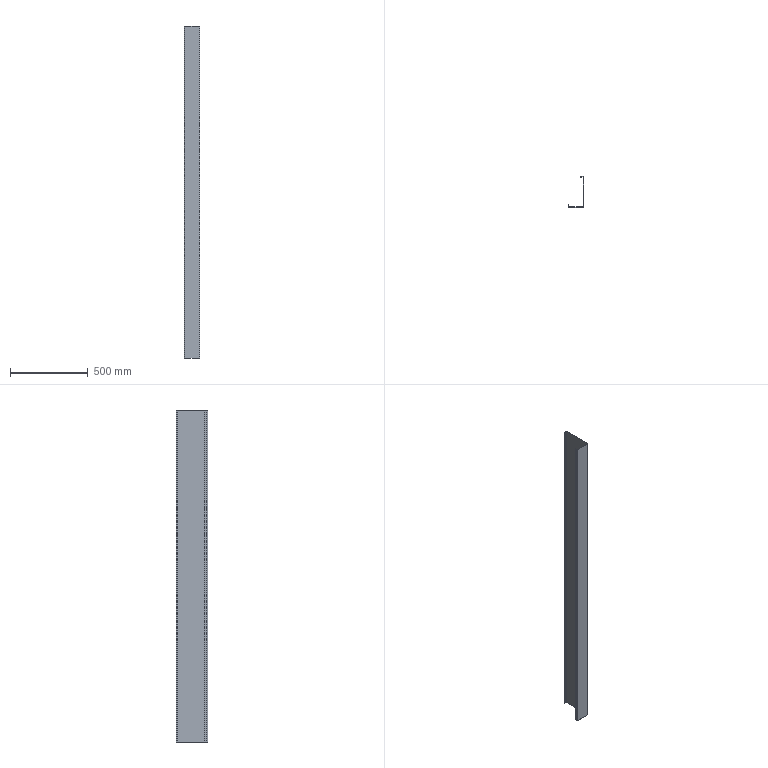Part | SolidWorks | features Extrusion 1, FlatPattern 1, SheetMetal 1, SolidToSheetMetal 1 | 1 solid | 30 faces | box 100 x 200 x 2130 mm | volume 1406384 mm3 | plane 24 | cylinder 6 | commonest cylinder face diameters 4 x3 8 x3
STEP:
#1=CARTESIAN_POINT('',(98.,196.,2130.));
#2=VERTEX_POINT('',#1);
#3=CARTESIAN_POINT('',(100.,196.,2130.));
#4=VERTEX_POINT('',#3);
#5=CARTESIAN_POINT('',(100.,196.,2130.));
#6=DIRECTION('',(1.,0.,0.));
#7=VECTOR('',#6,1000.);
#8=LINE('',#5,#7);
#9=EDGE_CURVE('',#2,#4,#8,.T.);
#10=ORIENTED_EDGE('',*,*,#9,.F.);
#11=CARTESIAN_POINT('',(98.,4.,2130.));
#12=VERTEX_POINT('',#11);
#13=CARTESIAN_POINT('',(98.,200.,2130.));
#14=DIRECTION('',(0.,1.,0.));
#15=VECTOR('',#14,1000.);
#16=LINE('',#13,#15);
#17=EDGE_CURVE('',#12,#2,#16,.T.);
#18=ORIENTED_EDGE('',*,*,#17,.F.);
#19=CARTESIAN_POINT('',(100.,4.,2130.));
#20=VERTEX_POINT('',#19);
#21=CARTESIAN_POINT('',(100.,4.,2130.));
#22=DIRECTION('',(1.,0.,0.));
#23=VECTOR('',#22,1000.);
#24=LINE('',#21,#23);
#25=EDGE_CURVE('',#12,#20,#24,.T.);
#26=ORIENTED_EDGE('',*,*,#25,.T.);
#27=CARTESIAN_POINT('',(100.,200.,2130.));
#28=DIRECTION('',(0.,1.,0.));
#29=VECTOR('',#28,1000.);
#30=LINE('',#27,#29);
#31=EDGE_CURVE('',#20,#4,#30,.T.);
#32=ORIENTED_EDGE('',*,*,#31,.T.);
#33=EDGE_LOOP('',(#10,#18,#26,#32));
#34=FACE_OUTER_BOUND('',#33,.T.);
#35=CARTESIAN_POINT('',(100.,200.,2130.));
#36=DIRECTION('',(0.,0.,1.));
#37=DIRECTION('',(0.,1.,0.));
#38=AXIS2_PLACEMENT_3D('',#35,#36,#37);
#39=PLANE('',#38);
#40=ADVANCED_FACE('',(#34),#39,.T.);
#41=ORIENTED_EDGE('',*,*,#25,.F.);
#42=CARTESIAN_POINT('',(96.,2.,2130.));
#43=VERTEX_POINT('',#42);
#44=CARTESIAN_POINT('',(96.,4.,2130.));
#45=DIRECTION('',(0.,0.,-1.));
#46=DIRECTION('',(-1.,0.,0.));
#47=AXIS2_PLACEMENT_3D('',#44,#45,#46);
#48=CIRCLE('',#47,2.);
#49=EDGE_CURVE('',#12,#43,#48,.T.);
#50=ORIENTED_EDGE('',*,*,#49,.T.);
#51=CARTESIAN_POINT('',(96.,0.,2130.));
#52=VERTEX_POINT('',#51);
#53=CARTESIAN_POINT('',(96.,0.,2130.));
#54=DIRECTION('',(0.,-1.,0.));
#55=VECTOR('',#54,1000.);
#56=LINE('',#53,#55);
#57=EDGE_CURVE('',#43,#52,#56,.T.);
#58=ORIENTED_EDGE('',*,*,#57,.T.);
#59=CARTESIAN_POINT('',(96.,4.,2130.));
#60=DIRECTION('',(0.,0.,-1.));
#61=DIRECTION('',(1.,0.,0.));
#62=AXIS2_PLACEMENT_3D('',#59,#60,#61);
#63=CIRCLE('',#62,4.);
#64=EDGE_CURVE('',#20,#52,#63,.T.);
#65=ORIENTED_EDGE('',*,*,#64,.F.);
#66=EDGE_LOOP('',(#41,#50,#58,#65));
#67=FACE_OUTER_BOUND('',#66,.T.);
#68=CARTESIAN_POINT('',(96.,4.,2130.));
#69=DIRECTION('',(0.,0.,-1.));
#70=DIRECTION('',(-1.,0.,0.));
#71=AXIS2_PLACEMENT_3D('',#68,#69,#70);
#72=PLANE('',#71);
#73=ADVANCED_FACE('',(#67),#72,.F.);
#74=ORIENTED_EDGE('',*,*,#57,.F.);
#75=CARTESIAN_POINT('',(4.,2.,2130.));
#76=VERTEX_POINT('',#75);
#77=CARTESIAN_POINT('',(100.,2.,2130.));
#78=DIRECTION('',(1.,0.,0.));
#79=VECTOR('',#78,1000.);
#80=LINE('',#77,#79);
#81=EDGE_CURVE('',#76,#43,#80,.T.);
#82=ORIENTED_EDGE('',*,*,#81,.F.);
#83=CARTESIAN_POINT('',(4.,0.,2130.));
#84=VERTEX_POINT('',#83);
#85=CARTESIAN_POINT('',(4.,0.,2130.));
#86=DIRECTION('',(0.,-1.,0.));
#87=VECTOR('',#86,1000.);
#88=LINE('',#85,#87);
#89=EDGE_CURVE('',#76,#84,#88,.T.);
#90=ORIENTED_EDGE('',*,*,#89,.T.);
#91=CARTESIAN_POINT('',(100.,0.,2130.));
#92=DIRECTION('',(1.,0.,0.));
#93=VECTOR('',#92,1000.);
#94=LINE('',#91,#93);
#95=EDGE_CURVE('',#84,#52,#94,.T.);
#96=ORIENTED_EDGE('',*,*,#95,.T.);
#97=EDGE_LOOP('',(#74,#82,#90,#96));
#98=FACE_OUTER_BOUND('',#97,.T.);
#99=CARTESIAN_POINT('',(100.,0.,2130.));
#100=DIRECTION('',(0.,0.,1.));
#101=DIRECTION('',(1.,0.,0.));
#102=AXIS2_PLACEMENT_3D('',#99,#100,#101);
#103=PLANE('',#102);
#104=ADVANCED_FACE('',(#98),#103,.T.);
#105=ORIENTED_EDGE('',*,*,#89,.F.);
#106=CARTESIAN_POINT('',(2.,4.,2130.));
#107=VERTEX_POINT('',#106);
#108=CARTESIAN_POINT('',(4.,4.,2130.));
#109=DIRECTION('',(0.,0.,-1.));
#110=DIRECTION('',(-1.,0.,0.));
#111=AXIS2_PLACEMENT_3D('',#108,#109,#110);
#112=CIRCLE('',#111,2.);
#113=EDGE_CURVE('',#76,#107,#112,.T.);
#114=ORIENTED_EDGE('',*,*,#113,.T.);
#115=CARTESIAN_POINT('',(0.,4.,2130.));
#116=VERTEX_POINT('',#115);
#117=CARTESIAN_POINT('',(0.,4.,2130.));
#118=DIRECTION('',(-1.,0.,0.));
#119=VECTOR('',#118,1000.);
#120=LINE('',#117,#119);
#121=EDGE_CURVE('',#107,#116,#120,.T.);
#122=ORIENTED_EDGE('',*,*,#121,.T.);
#123=CARTESIAN_POINT('',(4.,4.,2130.));
#124=DIRECTION('',(0.,0.,-1.));
#125=DIRECTION('',(1.,0.,0.));
#126=AXIS2_PLACEMENT_3D('',#123,#124,#125);
#127=CIRCLE('',#126,4.);
#128=EDGE_CURVE('',#84,#116,#127,.T.);
#129=ORIENTED_EDGE('',*,*,#128,.F.);
#130=EDGE_LOOP('',(#105,#114,#122,#129));
#131=FACE_OUTER_BOUND('',#130,.T.);
#132=CARTESIAN_POINT('',(4.,4.,2130.));
#133=DIRECTION('',(0.,0.,-1.));
#134=DIRECTION('',(-1.,0.,0.));
#135=AXIS2_PLACEMENT_3D('',#132,#133,#134);
#136=PLANE('',#135);
#137=ADVANCED_FACE('',(#131),#136,.F.);
#138=ORIENTED_EDGE('',*,*,#121,.F.);
#139=CARTESIAN_POINT('',(2.,20.,2130.));
#140=VERTEX_POINT('',#139);
#141=CARTESIAN_POINT('',(2.,0.,2130.));
#142=DIRECTION('',(0.,-1.,0.));
#143=VECTOR('',#142,1000.);
#144=LINE('',#141,#143);
#145=EDGE_CURVE('',#140,#107,#144,.T.);
#146=ORIENTED_EDGE('',*,*,#145,.F.);
#147=CARTESIAN_POINT('',(0.,20.,2130.));
#148=VERTEX_POINT('',#147);
#149=CARTESIAN_POINT('',(0.,20.,2130.));
#150=DIRECTION('',(-1.,0.,0.));
#151=VECTOR('',#150,1000.);
#152=LINE('',#149,#151);
#153=EDGE_CURVE('',#140,#148,#152,.T.);
#154=ORIENTED_EDGE('',*,*,#153,.T.);
#155=CARTESIAN_POINT('',(0.,0.,2130.));
#156=DIRECTION('',(0.,-1.,0.));
#157=VECTOR('',#156,1000.);
#158=LINE('',#155,#157);
#159=EDGE_CURVE('',#148,#116,#158,.T.);
#160=ORIENTED_EDGE('',*,*,#159,.T.);
#161=EDGE_LOOP('',(#138,#146,#154,#160));
#162=FACE_OUTER_BOUND('',#161,.T.);
#163=CARTESIAN_POINT('',(0.,0.,2130.));
#164=DIRECTION('',(0.,0.,1.));
#165=DIRECTION('',(0.,-1.,0.));
#166=AXIS2_PLACEMENT_3D('',#163,#164,#165);
#167=PLANE('',#166);
#168=ADVANCED_FACE('',(#162),#167,.T.);
#169=ORIENTED_EDGE('',*,*,#153,.F.);
#170=CARTESIAN_POINT('',(2.,20.,0.));
#171=VERTEX_POINT('',#170);
#172=CARTESIAN_POINT('',(2.,20.,2130.));
#173=DIRECTION('',(0.,0.,-1.));
#174=VECTOR('',#173,1000.);
#175=LINE('',#172,#174);
#176=EDGE_CURVE('',#140,#171,#175,.T.);
#177=ORIENTED_EDGE('',*,*,#176,.T.);
#178=CARTESIAN_POINT('',(0.,20.,0.));
#179=VERTEX_POINT('',#178);
#180=CARTESIAN_POINT('',(0.,20.,0.));
#181=DIRECTION('',(-1.,0.,0.));
#182=VECTOR('',#181,1000.);
#183=LINE('',#180,#182);
#184=EDGE_CURVE('',#171,#179,#183,.T.);
#185=ORIENTED_EDGE('',*,*,#184,.T.);
#186=CARTESIAN_POINT('',(0.,20.,2130.));
#187=DIRECTION('',(0.,0.,-1.));
#188=VECTOR('',#187,1000.);
#189=LINE('',#186,#188);
#190=EDGE_CURVE('',#148,#179,#189,.T.);
#191=ORIENTED_EDGE('',*,*,#190,.F.);
#192=EDGE_LOOP('',(#169,#177,#185,#191));
#193=FACE_OUTER_BOUND('',#192,.T.);
#194=CARTESIAN_POINT('',(0.,20.,2130.));
#195=DIRECTION('',(0.,-1.,0.));
#196=DIRECTION('',(0.,0.,-1.));
#197=AXIS2_PLACEMENT_3D('',#194,#195,#196);
#198=PLANE('',#197);
#199=ADVANCED_FACE('',(#193),#198,.F.);
#200=ORIENTED_EDGE('',*,*,#184,.F.);
#201=CARTESIAN_POINT('',(2.,4.,0.));
#202=VERTEX_POINT('',#201);
#203=CARTESIAN_POINT('',(2.,0.,0.));
#204=DIRECTION('',(0.,-1.,0.));
#205=VECTOR('',#204,1000.);
#206=LINE('',#203,#205);
#207=EDGE_CURVE('',#171,#202,#206,.T.);
#208=ORIENTED_EDGE('',*,*,#207,.T.);
#209=CARTESIAN_POINT('',(0.,4.,0.));
#210=VERTEX_POINT('',#209);
#211=CARTESIAN_POINT('',(0.,4.,0.));
#212=DIRECTION('',(-1.,0.,0.));
#213=VECTOR('',#212,1000.);
#214=LINE('',#211,#213);
#215=EDGE_CURVE('',#202,#210,#214,.T.);
#216=ORIENTED_EDGE('',*,*,#215,.T.);
#217=CARTESIAN_POINT('',(0.,0.,0.));
#218=DIRECTION('',(0.,-1.,0.));
#219=VECTOR('',#218,1000.);
#220=LINE('',#217,#219);
#221=EDGE_CURVE('',#179,#210,#220,.T.);
#222=ORIENTED_EDGE('',*,*,#221,.F.);
#223=EDGE_LOOP('',(#200,#208,#216,#222));
#224=FACE_OUTER_BOUND('',#223,.T.);
#225=CARTESIAN_POINT('',(0.,0.,0.));
#226=DIRECTION('',(0.,0.,1.));
#227=DIRECTION('',(0.,-1.,0.));
#228=AXIS2_PLACEMENT_3D('',#225,#226,#227);
#229=PLANE('',#228);
#230=ADVANCED_FACE('',(#224),#229,.F.);
#231=ORIENTED_EDGE('',*,*,#215,.F.);
#232=CARTESIAN_POINT('',(4.,2.,0.));
#233=VERTEX_POINT('',#232);
#234=CARTESIAN_POINT('',(4.,4.,0.));
#235=DIRECTION('',(0.,0.,1.));
#236=DIRECTION('',(-1.,0.,0.));
#237=AXIS2_PLACEMENT_3D('',#234,#235,#236);
#238=CIRCLE('',#237,2.);
#239=EDGE_CURVE('',#202,#233,#238,.T.);
#240=ORIENTED_EDGE('',*,*,#239,.T.);
#241=CARTESIAN_POINT('',(4.,0.,0.));
#242=VERTEX_POINT('',#241);
#243=CARTESIAN_POINT('',(4.,0.,0.));
#244=DIRECTION('',(0.,-1.,0.));
#245=VECTOR('',#244,1000.);
#246=LINE('',#243,#245);
#247=EDGE_CURVE('',#233,#242,#246,.T.);
#248=ORIENTED_EDGE('',*,*,#247,.T.);
#249=CARTESIAN_POINT('',(4.,4.,0.));
#250=DIRECTION('',(0.,0.,1.));
#251=DIRECTION('',(-1.,0.,0.));
#252=AXIS2_PLACEMENT_3D('',#249,#250,#251);
#253=CIRCLE('',#252,4.);
#254=EDGE_CURVE('',#210,#242,#253,.T.);
#255=ORIENTED_EDGE('',*,*,#254,.F.);
#256=EDGE_LOOP('',(#231,#240,#248,#255));
#257=FACE_OUTER_BOUND('',#256,.T.);
#258=CARTESIAN_POINT('',(4.,4.,0.));
#259=DIRECTION('',(0.,0.,1.));
#260=DIRECTION('',(1.,0.,0.));
#261=AXIS2_PLACEMENT_3D('',#258,#259,#260);
#262=PLANE('',#261);
#263=ADVANCED_FACE('',(#257),#262,.F.);
#264=ORIENTED_EDGE('',*,*,#247,.F.);
#265=CARTESIAN_POINT('',(96.,2.,0.));
#266=VERTEX_POINT('',#265);
#267=CARTESIAN_POINT('',(100.,2.,0.));
#268=DIRECTION('',(1.,0.,0.));
#269=VECTOR('',#268,1000.);
#270=LINE('',#267,#269);
#271=EDGE_CURVE('',#233,#266,#270,.T.);
#272=ORIENTED_EDGE('',*,*,#271,.T.);
#273=CARTESIAN_POINT('',(96.,0.,0.));
#274=VERTEX_POINT('',#273);
#275=CARTESIAN_POINT('',(96.,0.,0.));
#276=DIRECTION('',(0.,-1.,0.));
#277=VECTOR('',#276,1000.);
#278=LINE('',#275,#277);
#279=EDGE_CURVE('',#266,#274,#278,.T.);
#280=ORIENTED_EDGE('',*,*,#279,.T.);
#281=CARTESIAN_POINT('',(100.,0.,0.));
#282=DIRECTION('',(1.,0.,0.));
#283=VECTOR('',#282,1000.);
#284=LINE('',#281,#283);
#285=EDGE_CURVE('',#242,#274,#284,.T.);
#286=ORIENTED_EDGE('',*,*,#285,.F.);
#287=EDGE_LOOP('',(#264,#272,#280,#286));
#288=FACE_OUTER_BOUND('',#287,.T.);
#289=CARTESIAN_POINT('',(100.,0.,0.));
#290=DIRECTION('',(0.,0.,1.));
#291=DIRECTION('',(1.,0.,0.));
#292=AXIS2_PLACEMENT_3D('',#289,#290,#291);
#293=PLANE('',#292);
#294=ADVANCED_FACE('',(#288),#293,.F.);
#295=ORIENTED_EDGE('',*,*,#279,.F.);
#296=CARTESIAN_POINT('',(98.,4.,0.));
#297=VERTEX_POINT('',#296);
#298=CARTESIAN_POINT('',(96.,4.,0.));
#299=DIRECTION('',(0.,0.,1.));
#300=DIRECTION('',(-1.,0.,0.));
#301=AXIS2_PLACEMENT_3D('',#298,#299,#300);
#302=CIRCLE('',#301,2.);
#303=EDGE_CURVE('',#266,#297,#302,.T.);
#304=ORIENTED_EDGE('',*,*,#303,.T.);
#305=CARTESIAN_POINT('',(100.,4.,0.));
#306=VERTEX_POINT('',#305);
#307=CARTESIAN_POINT('',(100.,4.,0.));
#308=DIRECTION('',(1.,0.,0.));
#309=VECTOR('',#308,1000.);
#310=LINE('',#307,#309);
#311=EDGE_CURVE('',#297,#306,#310,.T.);
#312=ORIENTED_EDGE('',*,*,#311,.T.);
#313=CARTESIAN_POINT('',(96.,4.,0.));
#314=DIRECTION('',(0.,0.,1.));
#315=DIRECTION('',(-1.,0.,0.));
#316=AXIS2_PLACEMENT_3D('',#313,#314,#315);
#317=CIRCLE('',#316,4.);
#318=EDGE_CURVE('',#274,#306,#317,.T.);
#319=ORIENTED_EDGE('',*,*,#318,.F.);
#320=EDGE_LOOP('',(#295,#304,#312,#319));
#321=FACE_OUTER_BOUND('',#320,.T.);
#322=CARTESIAN_POINT('',(96.,4.,0.));
#323=DIRECTION('',(0.,0.,1.));
#324=DIRECTION('',(1.,0.,0.));
#325=AXIS2_PLACEMENT_3D('',#322,#323,#324);
#326=PLANE('',#325);
#327=ADVANCED_FACE('',(#321),#326,.F.);
#328=ORIENTED_EDGE('',*,*,#311,.F.);
#329=CARTESIAN_POINT('',(98.,196.,0.));
#330=VERTEX_POINT('',#329);
#331=CARTESIAN_POINT('',(98.,200.,0.));
#332=DIRECTION('',(0.,1.,0.));
#333=VECTOR('',#332,1000.);
#334=LINE('',#331,#333);
#335=EDGE_CURVE('',#297,#330,#334,.T.);
#336=ORIENTED_EDGE('',*,*,#335,.T.);
#337=CARTESIAN_POINT('',(100.,196.,0.));
#338=VERTEX_POINT('',#337);
#339=CARTESIAN_POINT('',(100.,196.,0.));
#340=DIRECTION('',(1.,0.,0.));
#341=VECTOR('',#340,1000.);
#342=LINE('',#339,#341);
#343=EDGE_CURVE('',#330,#338,#342,.T.);
#344=ORIENTED_EDGE('',*,*,#343,.T.);
#345=CARTESIAN_POINT('',(100.,200.,0.));
#346=DIRECTION('',(0.,1.,0.));
#347=VECTOR('',#346,1000.);
#348=LINE('',#345,#347);
#349=EDGE_CURVE('',#306,#338,#348,.T.);
#350=ORIENTED_EDGE('',*,*,#349,.F.);
#351=EDGE_LOOP('',(#328,#336,#344,#350));
#352=FACE_OUTER_BOUND('',#351,.T.);
#353=CARTESIAN_POINT('',(100.,200.,0.));
#354=DIRECTION('',(0.,0.,1.));
#355=DIRECTION('',(0.,1.,0.));
#356=AXIS2_PLACEMENT_3D('',#353,#354,#355);
#357=PLANE('',#356);
#358=ADVANCED_FACE('',(#352),#357,.F.);
#359=ORIENTED_EDGE('',*,*,#343,.F.);
#360=CARTESIAN_POINT('',(96.,198.,0.));
#361=VERTEX_POINT('',#360);
#362=CARTESIAN_POINT('',(96.,196.,0.));
#363=DIRECTION('',(0.,0.,1.));
#364=DIRECTION('',(-1.,0.,0.));
#365=AXIS2_PLACEMENT_3D('',#362,#363,#364);
#366=CIRCLE('',#365,2.);
#367=EDGE_CURVE('',#330,#361,#366,.T.);
#368=ORIENTED_EDGE('',*,*,#367,.T.);
#369=CARTESIAN_POINT('',(96.,200.,0.));
#370=VERTEX_POINT('',#369);
#371=CARTESIAN_POINT('',(96.,200.,0.));
#372=DIRECTION('',(0.,1.,0.));
#373=VECTOR('',#372,1000.);
#374=LINE('',#371,#373);
#375=EDGE_CURVE('',#361,#370,#374,.T.);
#376=ORIENTED_EDGE('',*,*,#375,.T.);
#377=CARTESIAN_POINT('',(96.,196.,0.));
#378=DIRECTION('',(0.,0.,1.));
#379=DIRECTION('',(-1.,0.,0.));
#380=AXIS2_PLACEMENT_3D('',#377,#378,#379);
#381=CIRCLE('',#380,4.);
#382=EDGE_CURVE('',#338,#370,#381,.T.);
#383=ORIENTED_EDGE('',*,*,#382,.F.);
#384=EDGE_LOOP('',(#359,#368,#376,#383));
#385=FACE_OUTER_BOUND('',#384,.T.);
#386=CARTESIAN_POINT('',(96.,196.,0.));
#387=DIRECTION('',(0.,0.,1.));
#388=DIRECTION('',(1.,0.,0.));
#389=AXIS2_PLACEMENT_3D('',#386,#387,#388);
#390=PLANE('',#389);
#391=ADVANCED_FACE('',(#385),#390,.F.);
#392=ORIENTED_EDGE('',*,*,#375,.F.);
#393=CARTESIAN_POINT('',(80.,198.,0.));
#394=VERTEX_POINT('',#393);
#395=CARTESIAN_POINT('',(80.,198.,0.));
#396=DIRECTION('',(-1.,0.,0.));
#397=VECTOR('',#396,1000.);
#398=LINE('',#395,#397);
#399=EDGE_CURVE('',#361,#394,#398,.T.);
#400=ORIENTED_EDGE('',*,*,#399,.T.);
#401=CARTESIAN_POINT('',(80.,200.,0.));
#402=VERTEX_POINT('',#401);
#403=CARTESIAN_POINT('',(80.,200.,0.));
#404=DIRECTION('',(0.,1.,0.));
#405=VECTOR('',#404,1000.);
#406=LINE('',#403,#405);
#407=EDGE_CURVE('',#394,#402,#406,.T.);
#408=ORIENTED_EDGE('',*,*,#407,.T.);
#409=CARTESIAN_POINT('',(80.,200.,0.));
#410=DIRECTION('',(-1.,0.,0.));
#411=VECTOR('',#410,1000.);
#412=LINE('',#409,#411);
#413=EDGE_CURVE('',#370,#402,#412,.T.);
#414=ORIENTED_EDGE('',*,*,#413,.F.);
#415=EDGE_LOOP('',(#392,#400,#408,#414));
#416=FACE_OUTER_BOUND('',#415,.T.);
#417=CARTESIAN_POINT('',(80.,200.,0.));
#418=DIRECTION('',(0.,0.,1.));
#419=DIRECTION('',(-1.,0.,0.));
#420=AXIS2_PLACEMENT_3D('',#417,#418,#419);
#421=PLANE('',#420);
#422=ADVANCED_FACE('',(#416),#421,.F.);
#423=ORIENTED_EDGE('',*,*,#407,.F.);
#424=CARTESIAN_POINT('',(80.,198.,2130.));
#425=VERTEX_POINT('',#424);
#426=CARTESIAN_POINT('',(80.,198.,2130.));
#427=DIRECTION('',(0.,0.,-1.));
#428=VECTOR('',#427,1000.);
#429=LINE('',#426,#428);
#430=EDGE_CURVE('',#425,#394,#429,.T.);
#431=ORIENTED_EDGE('',*,*,#430,.F.);
#432=CARTESIAN_POINT('',(80.,200.,2130.));
#433=VERTEX_POINT('',#432);
#434=CARTESIAN_POINT('',(80.,200.,2130.));
#435=DIRECTION('',(0.,1.,0.));
#436=VECTOR('',#435,1000.);
#437=LINE('',#434,#436);
#438=EDGE_CURVE('',#425,#433,#437,.T.);
#439=ORIENTED_EDGE('',*,*,#438,.T.);
#440=CARTESIAN_POINT('',(80.,200.,2130.));
#441=DIRECTION('',(0.,0.,-1.));
#442=VECTOR('',#441,1000.);
#443=LINE('',#440,#442);
#444=EDGE_CURVE('',#433,#402,#443,.T.);
#445=ORIENTED_EDGE('',*,*,#444,.T.);
#446=EDGE_LOOP('',(#423,#431,#439,#445));
#447=FACE_OUTER_BOUND('',#446,.T.);
#448=CARTESIAN_POINT('',(80.,200.,2130.));
#449=DIRECTION('',(-1.,0.,0.));
#450=DIRECTION('',(0.,0.,-1.));
#451=AXIS2_PLACEMENT_3D('',#448,#449,#450);
#452=PLANE('',#451);
#453=ADVANCED_FACE('',(#447),#452,.T.);
#454=ORIENTED_EDGE('',*,*,#438,.F.);
#455=CARTESIAN_POINT('',(96.,198.,2130.));
#456=VERTEX_POINT('',#455);
#457=CARTESIAN_POINT('',(80.,198.,2130.));
#458=DIRECTION('',(-1.,0.,0.));
#459=VECTOR('',#458,1000.);
#460=LINE('',#457,#459);
#461=EDGE_CURVE('',#456,#425,#460,.T.);
#462=ORIENTED_EDGE('',*,*,#461,.F.);
#463=CARTESIAN_POINT('',(96.,200.,2130.));
#464=VERTEX_POINT('',#463);
#465=CARTESIAN_POINT('',(96.,200.,2130.));
#466=DIRECTION('',(0.,1.,0.));
#467=VECTOR('',#466,1000.);
#468=LINE('',#465,#467);
#469=EDGE_CURVE('',#456,#464,#468,.T.);
#470=ORIENTED_EDGE('',*,*,#469,.T.);
#471=CARTESIAN_POINT('',(80.,200.,2130.));
#472=DIRECTION('',(-1.,0.,0.));
#473=VECTOR('',#472,1000.);
#474=LINE('',#471,#473);
#475=EDGE_CURVE('',#464,#433,#474,.T.);
#476=ORIENTED_EDGE('',*,*,#475,.T.);
#477=EDGE_LOOP('',(#454,#462,#470,#476));
#478=FACE_OUTER_BOUND('',#477,.T.);
#479=CARTESIAN_POINT('',(80.,200.,2130.));
#480=DIRECTION('',(0.,0.,1.));
#481=DIRECTION('',(-1.,0.,0.));
#482=AXIS2_PLACEMENT_3D('',#479,#480,#481);
#483=PLANE('',#482);
#484=ADVANCED_FACE('',(#478),#483,.T.);
#485=CARTESIAN_POINT('',(96.,196.,2130.));
#486=DIRECTION('',(0.,0.,-1.));
#487=DIRECTION('',(-1.,0.,0.));
#488=AXIS2_PLACEMENT_3D('',#485,#486,#487);
#489=CIRCLE('',#488,2.);
#490=EDGE_CURVE('',#456,#2,#489,.T.);
#491=ORIENTED_EDGE('',*,*,#490,.T.);
#492=ORIENTED_EDGE('',*,*,#9,.T.);
#493=CARTESIAN_POINT('',(96.,196.,2130.));
#494=DIRECTION('',(0.,0.,-1.));
#495=DIRECTION('',(1.,0.,0.));
#496=AXIS2_PLACEMENT_3D('',#493,#494,#495);
#497=CIRCLE('',#496,4.);
#498=EDGE_CURVE('',#464,#4,#497,.T.);
#499=ORIENTED_EDGE('',*,*,#498,.F.);
#500=ORIENTED_EDGE('',*,*,#469,.F.);
#501=EDGE_LOOP('',(#491,#492,#499,#500));
#502=FACE_OUTER_BOUND('',#501,.T.);
#503=CARTESIAN_POINT('',(96.,196.,2130.));
#504=DIRECTION('',(0.,0.,-1.));
#505=DIRECTION('',(-1.,0.,0.));
#506=AXIS2_PLACEMENT_3D('',#503,#504,#505);
#507=PLANE('',#506);
#508=ADVANCED_FACE('',(#502),#507,.F.);
#509=ORIENTED_EDGE('',*,*,#475,.F.);
#510=CARTESIAN_POINT('',(96.,200.,2130.));
#511=DIRECTION('',(0.,0.,-1.));
#512=VECTOR('',#511,1000.);
#513=LINE('',#510,#512);
#514=EDGE_CURVE('',#464,#370,#513,.T.);
#515=ORIENTED_EDGE('',*,*,#514,.T.);
#516=ORIENTED_EDGE('',*,*,#413,.T.);
#517=ORIENTED_EDGE('',*,*,#444,.F.);
#518=EDGE_LOOP('',(#509,#515,#516,#517));
#519=FACE_OUTER_BOUND('',#518,.T.);
#520=CARTESIAN_POINT('',(80.,200.,2130.));
#521=DIRECTION('',(0.,-1.,0.));
#522=DIRECTION('',(0.,0.,-1.));
#523=AXIS2_PLACEMENT_3D('',#520,#521,#522);
#524=PLANE('',#523);
#525=ADVANCED_FACE('',(#519),#524,.F.);
#526=ORIENTED_EDGE('',*,*,#221,.T.);
#527=CARTESIAN_POINT('',(0.,4.,2130.));
#528=DIRECTION('',(0.,0.,1.));
#529=VECTOR('',#528,1000.);
#530=LINE('',#527,#529);
#531=EDGE_CURVE('',#210,#116,#530,.T.);
#532=ORIENTED_EDGE('',*,*,#531,.T.);
#533=ORIENTED_EDGE('',*,*,#159,.F.);
#534=ORIENTED_EDGE('',*,*,#190,.T.);
#535=EDGE_LOOP('',(#526,#532,#533,#534));
#536=FACE_OUTER_BOUND('',#535,.T.);
#537=CARTESIAN_POINT('',(0.,0.,2130.));
#538=DIRECTION('',(1.,0.,0.));
#539=DIRECTION('',(0.,0.,-1.));
#540=AXIS2_PLACEMENT_3D('',#537,#538,#539);
#541=PLANE('',#540);
#542=ADVANCED_FACE('',(#536),#541,.F.);
#543=ORIENTED_EDGE('',*,*,#285,.T.);
#544=CARTESIAN_POINT('',(96.,0.,2130.));
#545=DIRECTION('',(0.,0.,1.));
#546=VECTOR('',#545,1000.);
#547=LINE('',#544,#546);
#548=EDGE_CURVE('',#274,#52,#547,.T.);
#549=ORIENTED_EDGE('',*,*,#548,.T.);
#550=ORIENTED_EDGE('',*,*,#95,.F.);
#551=CARTESIAN_POINT('',(4.,0.,2130.));
#552=DIRECTION('',(0.,0.,-1.));
#553=VECTOR('',#552,1000.);
#554=LINE('',#551,#553);
#555=EDGE_CURVE('',#84,#242,#554,.T.);
#556=ORIENTED_EDGE('',*,*,#555,.T.);
#557=EDGE_LOOP('',(#543,#549,#550,#556));
#558=FACE_OUTER_BOUND('',#557,.T.);
#559=CARTESIAN_POINT('',(100.,0.,2130.));
#560=DIRECTION('',(0.,1.,0.));
#561=DIRECTION('',(0.,0.,1.));
#562=AXIS2_PLACEMENT_3D('',#559,#560,#561);
#563=PLANE('',#562);
#564=ADVANCED_FACE('',(#558),#563,.F.);
#565=ORIENTED_EDGE('',*,*,#349,.T.);
#566=CARTESIAN_POINT('',(100.,196.,2130.));
#567=DIRECTION('',(0.,0.,1.));
#568=VECTOR('',#567,1000.);
#569=LINE('',#566,#568);
#570=EDGE_CURVE('',#338,#4,#569,.T.);
#571=ORIENTED_EDGE('',*,*,#570,.T.);
#572=ORIENTED_EDGE('',*,*,#31,.F.);
#573=CARTESIAN_POINT('',(100.,4.,2130.));
#574=DIRECTION('',(0.,0.,-1.));
#575=VECTOR('',#574,1000.);
#576=LINE('',#573,#575);
#577=EDGE_CURVE('',#20,#306,#576,.T.);
#578=ORIENTED_EDGE('',*,*,#577,.T.);
#579=EDGE_LOOP('',(#565,#571,#572,#578));
#580=FACE_OUTER_BOUND('',#579,.T.);
#581=CARTESIAN_POINT('',(100.,200.,2130.));
#582=DIRECTION('',(-1.,0.,0.));
#583=DIRECTION('',(0.,0.,1.));
#584=AXIS2_PLACEMENT_3D('',#581,#582,#583);
#585=PLANE('',#584);
#586=ADVANCED_FACE('',(#580),#585,.F.);
#587=ORIENTED_EDGE('',*,*,#128,.T.);
#588=ORIENTED_EDGE('',*,*,#531,.F.);
#589=ORIENTED_EDGE('',*,*,#254,.T.);
#590=ORIENTED_EDGE('',*,*,#555,.F.);
#591=EDGE_LOOP('',(#587,#588,#589,#590));
#592=FACE_OUTER_BOUND('',#591,.T.);
#593=CARTESIAN_POINT('',(4.,4.,2130.));
#594=DIRECTION('',(0.,0.,-1.));
#595=DIRECTION('',(-1.,0.,0.));
#596=AXIS2_PLACEMENT_3D('',#593,#594,#595);
#597=CYLINDRICAL_SURFACE('',#596,4.);
#598=ADVANCED_FACE('',(#592),#597,.T.);
#599=ORIENTED_EDGE('',*,*,#64,.T.);
#600=ORIENTED_EDGE('',*,*,#548,.F.);
#601=ORIENTED_EDGE('',*,*,#318,.T.);
#602=ORIENTED_EDGE('',*,*,#577,.F.);
#603=EDGE_LOOP('',(#599,#600,#601,#602));
#604=FACE_OUTER_BOUND('',#603,.T.);
#605=CARTESIAN_POINT('',(96.,4.,2130.));
#606=DIRECTION('',(0.,0.,-1.));
#607=DIRECTION('',(-1.,0.,0.));
#608=AXIS2_PLACEMENT_3D('',#605,#606,#607);
#609=CYLINDRICAL_SURFACE('',#608,4.);
#610=ADVANCED_FACE('',(#604),#609,.T.);
#611=ORIENTED_EDGE('',*,*,#498,.T.);
#612=ORIENTED_EDGE('',*,*,#570,.F.);
#613=ORIENTED_EDGE('',*,*,#382,.T.);
#614=ORIENTED_EDGE('',*,*,#514,.F.);
#615=EDGE_LOOP('',(#611,#612,#613,#614));
#616=FACE_OUTER_BOUND('',#615,.T.);
#617=CARTESIAN_POINT('',(96.,196.,2130.));
#618=DIRECTION('',(0.,0.,-1.));
#619=DIRECTION('',(-1.,0.,0.));
#620=AXIS2_PLACEMENT_3D('',#617,#618,#619);
#621=CYLINDRICAL_SURFACE('',#620,4.);
#622=ADVANCED_FACE('',(#616),#621,.T.);
#623=ORIENTED_EDGE('',*,*,#461,.T.);
#624=ORIENTED_EDGE('',*,*,#430,.T.);
#625=ORIENTED_EDGE('',*,*,#399,.F.);
#626=CARTESIAN_POINT('',(96.,198.,2130.));
#627=DIRECTION('',(0.,0.,-1.));
#628=VECTOR('',#627,1000.);
#629=LINE('',#626,#628);
#630=EDGE_CURVE('',#456,#361,#629,.T.);
#631=ORIENTED_EDGE('',*,*,#630,.F.);
#632=EDGE_LOOP('',(#623,#624,#625,#631));
#633=FACE_OUTER_BOUND('',#632,.T.);
#634=CARTESIAN_POINT('',(80.,198.,2130.));
#635=DIRECTION('',(0.,-1.,0.));
#636=DIRECTION('',(0.,0.,-1.));
#637=AXIS2_PLACEMENT_3D('',#634,#635,#636);
#638=PLANE('',#637);
#639=ADVANCED_FACE('',(#633),#638,.T.);
#640=ORIENTED_EDGE('',*,*,#207,.F.);
#641=ORIENTED_EDGE('',*,*,#176,.F.);
#642=ORIENTED_EDGE('',*,*,#145,.T.);
#643=CARTESIAN_POINT('',(2.,4.,2130.));
#644=DIRECTION('',(0.,0.,1.));
#645=VECTOR('',#644,1000.);
#646=LINE('',#643,#645);
#647=EDGE_CURVE('',#202,#107,#646,.T.);
#648=ORIENTED_EDGE('',*,*,#647,.F.);
#649=EDGE_LOOP('',(#640,#641,#642,#648));
#650=FACE_OUTER_BOUND('',#649,.T.);
#651=CARTESIAN_POINT('',(2.,0.,2130.));
#652=DIRECTION('',(1.,0.,0.));
#653=DIRECTION('',(0.,0.,-1.));
#654=AXIS2_PLACEMENT_3D('',#651,#652,#653);
#655=PLANE('',#654);
#656=ADVANCED_FACE('',(#650),#655,.T.);
#657=ORIENTED_EDGE('',*,*,#271,.F.);
#658=CARTESIAN_POINT('',(4.,2.,2130.));
#659=DIRECTION('',(0.,0.,-1.));
#660=VECTOR('',#659,1000.);
#661=LINE('',#658,#660);
#662=EDGE_CURVE('',#76,#233,#661,.T.);
#663=ORIENTED_EDGE('',*,*,#662,.F.);
#664=ORIENTED_EDGE('',*,*,#81,.T.);
#665=CARTESIAN_POINT('',(96.,2.,2130.));
#666=DIRECTION('',(0.,0.,1.));
#667=VECTOR('',#666,1000.);
#668=LINE('',#665,#667);
#669=EDGE_CURVE('',#266,#43,#668,.T.);
#670=ORIENTED_EDGE('',*,*,#669,.F.);
#671=EDGE_LOOP('',(#657,#663,#664,#670));
#672=FACE_OUTER_BOUND('',#671,.T.);
#673=CARTESIAN_POINT('',(100.,2.,2130.));
#674=DIRECTION('',(0.,1.,0.));
#675=DIRECTION('',(0.,0.,1.));
#676=AXIS2_PLACEMENT_3D('',#673,#674,#675);
#677=PLANE('',#676);
#678=ADVANCED_FACE('',(#672),#677,.T.);
#679=ORIENTED_EDGE('',*,*,#335,.F.);
#680=CARTESIAN_POINT('',(98.,4.,2130.));
#681=DIRECTION('',(0.,0.,-1.));
#682=VECTOR('',#681,1000.);
#683=LINE('',#680,#682);
#684=EDGE_CURVE('',#12,#297,#683,.T.);
#685=ORIENTED_EDGE('',*,*,#684,.F.);
#686=ORIENTED_EDGE('',*,*,#17,.T.);
#687=CARTESIAN_POINT('',(98.,196.,2130.));
#688=DIRECTION('',(0.,0.,1.));
#689=VECTOR('',#688,1000.);
#690=LINE('',#687,#689);
#691=EDGE_CURVE('',#330,#2,#690,.T.);
#692=ORIENTED_EDGE('',*,*,#691,.F.);
#693=EDGE_LOOP('',(#679,#685,#686,#692));
#694=FACE_OUTER_BOUND('',#693,.T.);
#695=CARTESIAN_POINT('',(98.,200.,2130.));
#696=DIRECTION('',(-1.,0.,0.));
#697=DIRECTION('',(0.,0.,1.));
#698=AXIS2_PLACEMENT_3D('',#695,#696,#697);
#699=PLANE('',#698);
#700=ADVANCED_FACE('',(#694),#699,.T.);
#701=ORIENTED_EDGE('',*,*,#113,.F.);
#702=ORIENTED_EDGE('',*,*,#662,.T.);
#703=ORIENTED_EDGE('',*,*,#239,.F.);
#704=ORIENTED_EDGE('',*,*,#647,.T.);
#705=EDGE_LOOP('',(#701,#702,#703,#704));
#706=FACE_OUTER_BOUND('',#705,.T.);
#707=CARTESIAN_POINT('',(4.,4.,2130.));
#708=DIRECTION('',(0.,0.,-1.));
#709=DIRECTION('',(-1.,0.,0.));
#710=AXIS2_PLACEMENT_3D('',#707,#708,#709);
#711=CYLINDRICAL_SURFACE('',#710,2.);
#712=ADVANCED_FACE('',(#706),#711,.F.);
#713=ORIENTED_EDGE('',*,*,#49,.F.);
#714=ORIENTED_EDGE('',*,*,#684,.T.);
#715=ORIENTED_EDGE('',*,*,#303,.F.);
#716=ORIENTED_EDGE('',*,*,#669,.T.);
#717=EDGE_LOOP('',(#713,#714,#715,#716));
#718=FACE_OUTER_BOUND('',#717,.T.);
#719=CARTESIAN_POINT('',(96.,4.,2130.));
#720=DIRECTION('',(0.,0.,-1.));
#721=DIRECTION('',(-1.,0.,0.));
#722=AXIS2_PLACEMENT_3D('',#719,#720,#721);
#723=CYLINDRICAL_SURFACE('',#722,2.);
#724=ADVANCED_FACE('',(#718),#723,.F.);
#725=ORIENTED_EDGE('',*,*,#490,.F.);
#726=ORIENTED_EDGE('',*,*,#630,.T.);
#727=ORIENTED_EDGE('',*,*,#367,.F.);
#728=ORIENTED_EDGE('',*,*,#691,.T.);
#729=EDGE_LOOP('',(#725,#726,#727,#728));
#730=FACE_OUTER_BOUND('',#729,.T.);
#731=CARTESIAN_POINT('',(96.,196.,2130.));
#732=DIRECTION('',(0.,0.,-1.));
#733=DIRECTION('',(-1.,0.,0.));
#734=AXIS2_PLACEMENT_3D('',#731,#732,#733);
#735=CYLINDRICAL_SURFACE('',#734,2.);
#736=ADVANCED_FACE('',(#730),#735,.F.);
#737=CLOSED_SHELL('',(#40,#73,#104,#137,#168,#199,#230,#263,#294,#327,#358,#391,#422,#453,#484,#508,#525,#542,#564,#586,#598,#610,#622,#639,#656,#678,#700,#712,#724,#736));
#738=MANIFOLD_SOLID_BREP('',#737);
#739=CARTESIAN_POINT('',(0.,0.,0.));
#740=DIRECTION('',(0.,0.,1.));
#741=DIRECTION('',(1.,0.,0.));
#742=AXIS2_PLACEMENT_3D('',#739,#740,#741);
#743=(LENGTH_UNIT()NAMED_UNIT(*)SI_UNIT(.MILLI.,.METRE.));
#744=UNCERTAINTY_MEASURE_WITH_UNIT(LENGTH_MEASURE(0.00001),#743,'','');
#745=(NAMED_UNIT(*)PLANE_ANGLE_UNIT()SI_UNIT($,.RADIAN.));
#746=(NAMED_UNIT(*)SI_UNIT($,.STERADIAN.)SOLID_ANGLE_UNIT());
#747=(GEOMETRIC_REPRESENTATION_CONTEXT(3)GLOBAL_UNCERTAINTY_ASSIGNED_CONTEXT((#744))GLOBAL_UNIT_ASSIGNED_CONTEXT((#743,#745,#746))REPRESENTATION_CONTEXT('',''));
#748=ADVANCED_BREP_SHAPE_REPRESENTATION('',(#738,#742),#747);